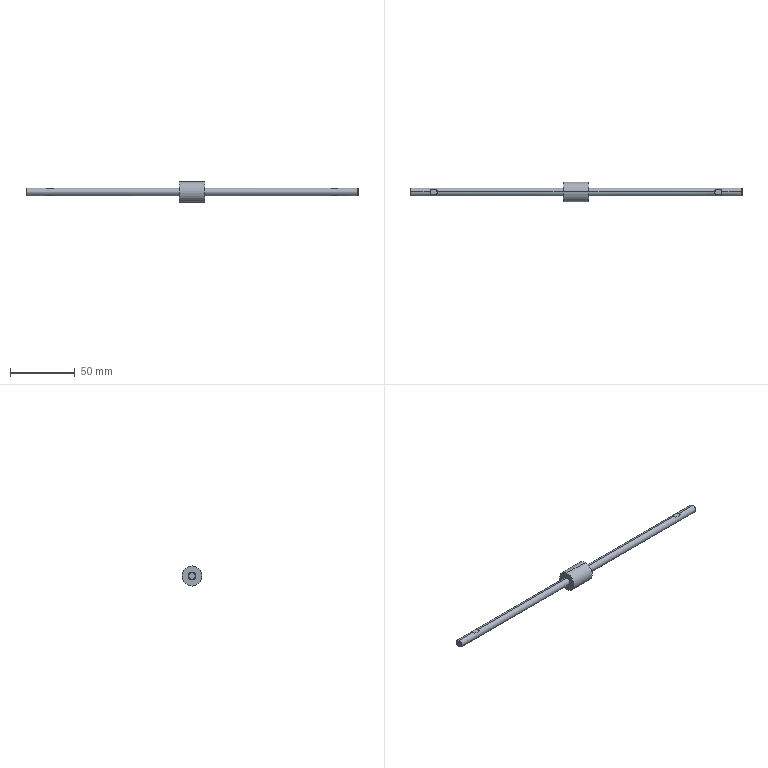Part | STEP file | _16MAD600Rod | 1 solid | 26 faces | box 256 x 15.5 x 15.5 mm | volume 10417 mm3 | plane 16 | cylinder 6 | cone 4 | commonest cylinder face diameters 6 x4 15.5 x2
STEP:
#1=CARTESIAN_POINT('',(118.,0.,3.));
#2=VERTEX_POINT('',#1);
#3=CARTESIAN_POINT('',(118.,0.,-3.));
#4=VERTEX_POINT('',#3);
#5=CARTESIAN_POINT('',(118.,0.,0.));
#6=DIRECTION('',(-1.,0.,0.));
#7=DIRECTION('',(0.,0.,1.));
#8=AXIS2_PLACEMENT_3D('',#5,#6,#7);
#9=CIRCLE('',#8,3.);
#10=EDGE_CURVE('',#2,#4,#9,.T.);
#11=ORIENTED_EDGE('',*,*,#10,.T.);
#12=CARTESIAN_POINT('',(21.3,0.,-3.));
#13=VERTEX_POINT('',#12);
#14=CARTESIAN_POINT('',(256.,0.,-3.));
#15=DIRECTION('',(-1.,0.,0.));
#16=VECTOR('',#15,1000.);
#17=LINE('',#14,#16);
#18=EDGE_CURVE('',#4,#13,#17,.T.);
#19=ORIENTED_EDGE('',*,*,#18,.T.);
#20=CARTESIAN_POINT('',(20.8,1.658,-2.5));
#21=VERTEX_POINT('',#20);
#22=CARTESIAN_POINT('',(21.3,0.,-3.));
#23=CARTESIAN_POINT('',(21.3,0.5942,-3.));
#24=CARTESIAN_POINT('',(21.128,1.163,-2.828));
#25=CARTESIAN_POINT('',(20.8,1.658,-2.5));
#26=(BOUNDED_CURVE()B_SPLINE_CURVE(3,(#22,#23,#24,#25),.UNSPECIFIED.,.F.,.F.)B_SPLINE_CURVE_WITH_KNOTS((4,4),(3.142,3.727),.UNSPECIFIED.)CURVE()GEOMETRIC_REPRESENTATION_ITEM()RATIONAL_B_SPLINE_CURVE((1.,0.9716,0.9716,1.))REPRESENTATION_ITEM(''));
#27=EDGE_CURVE('',#13,#21,#26,.T.);
#28=ORIENTED_EDGE('',*,*,#27,.T.);
#29=CARTESIAN_POINT('',(16.,1.658,-2.5));
#30=VERTEX_POINT('',#29);
#31=CARTESIAN_POINT('',(256.,1.658,-2.5));
#32=DIRECTION('',(-1.,0.,0.));
#33=VECTOR('',#32,1000.);
#34=LINE('',#31,#33);
#35=EDGE_CURVE('',#21,#30,#34,.T.);
#36=ORIENTED_EDGE('',*,*,#35,.T.);
#37=CARTESIAN_POINT('',(15.5,0.,-3.));
#38=VERTEX_POINT('',#37);
#39=CARTESIAN_POINT('',(16.,1.658,-2.5));
#40=CARTESIAN_POINT('',(15.672,1.163,-2.828));
#41=CARTESIAN_POINT('',(15.5,0.5942,-3.));
#42=CARTESIAN_POINT('',(15.5,0.,-3.));
#43=(BOUNDED_CURVE()B_SPLINE_CURVE(3,(#39,#40,#41,#42),.UNSPECIFIED.,.F.,.F.)B_SPLINE_CURVE_WITH_KNOTS((4,4),(5.697,6.283),.UNSPECIFIED.)CURVE()GEOMETRIC_REPRESENTATION_ITEM()RATIONAL_B_SPLINE_CURVE((1.,0.9716,0.9716,1.))REPRESENTATION_ITEM(''));
#44=EDGE_CURVE('',#30,#38,#43,.T.);
#45=ORIENTED_EDGE('',*,*,#44,.T.);
#46=CARTESIAN_POINT('',(0.6135,0.,-3.));
#47=VERTEX_POINT('',#46);
#48=CARTESIAN_POINT('',(256.,0.,-3.));
#49=DIRECTION('',(-1.,0.,0.));
#50=VECTOR('',#49,1000.);
#51=LINE('',#48,#50);
#52=EDGE_CURVE('',#38,#47,#51,.T.);
#53=ORIENTED_EDGE('',*,*,#52,.T.);
#54=CARTESIAN_POINT('',(0.6135,0.,3.));
#55=VERTEX_POINT('',#54);
#56=CARTESIAN_POINT('',(0.6135,0.,0.));
#57=DIRECTION('',(1.,0.,0.));
#58=DIRECTION('',(0.,0.,1.));
#59=AXIS2_PLACEMENT_3D('',#56,#57,#58);
#60=CIRCLE('',#59,3.);
#61=EDGE_CURVE('',#47,#55,#60,.T.);
#62=ORIENTED_EDGE('',*,*,#61,.T.);
#63=CARTESIAN_POINT('',(15.5,0.,3.));
#64=VERTEX_POINT('',#63);
#65=CARTESIAN_POINT('',(256.,0.,3.));
#66=DIRECTION('',(-1.,0.,0.));
#67=VECTOR('',#66,1000.);
#68=LINE('',#65,#67);
#69=EDGE_CURVE('',#64,#55,#68,.T.);
#70=ORIENTED_EDGE('',*,*,#69,.F.);
#71=CARTESIAN_POINT('',(16.,1.658,2.5));
#72=VERTEX_POINT('',#71);
#73=CARTESIAN_POINT('',(15.5,0.,3.));
#74=CARTESIAN_POINT('',(15.5,0.5942,3.));
#75=CARTESIAN_POINT('',(15.672,1.163,2.828));
#76=CARTESIAN_POINT('',(16.,1.658,2.5));
#77=(BOUNDED_CURVE()B_SPLINE_CURVE(3,(#73,#74,#75,#76),.UNSPECIFIED.,.F.,.F.)B_SPLINE_CURVE_WITH_KNOTS((4,4),(0.,0.5857),.UNSPECIFIED.)CURVE()GEOMETRIC_REPRESENTATION_ITEM()RATIONAL_B_SPLINE_CURVE((1.,0.9716,0.9716,1.))REPRESENTATION_ITEM(''));
#78=EDGE_CURVE('',#64,#72,#77,.T.);
#79=ORIENTED_EDGE('',*,*,#78,.T.);
#80=CARTESIAN_POINT('',(20.8,1.658,2.5));
#81=VERTEX_POINT('',#80);
#82=CARTESIAN_POINT('',(256.,1.658,2.5));
#83=DIRECTION('',(1.,0.,0.));
#84=VECTOR('',#83,1000.);
#85=LINE('',#82,#84);
#86=EDGE_CURVE('',#72,#81,#85,.T.);
#87=ORIENTED_EDGE('',*,*,#86,.T.);
#88=CARTESIAN_POINT('',(21.3,0.,3.));
#89=VERTEX_POINT('',#88);
#90=CARTESIAN_POINT('',(20.8,1.658,2.5));
#91=CARTESIAN_POINT('',(21.128,1.163,2.828));
#92=CARTESIAN_POINT('',(21.3,0.5942,3.));
#93=CARTESIAN_POINT('',(21.3,0.,3.));
#94=(BOUNDED_CURVE()B_SPLINE_CURVE(3,(#90,#91,#92,#93),.UNSPECIFIED.,.F.,.F.)B_SPLINE_CURVE_WITH_KNOTS((4,4),(2.556,3.142),.UNSPECIFIED.)CURVE()GEOMETRIC_REPRESENTATION_ITEM()RATIONAL_B_SPLINE_CURVE((1.,0.9716,0.9716,1.))REPRESENTATION_ITEM(''));
#95=EDGE_CURVE('',#81,#89,#94,.T.);
#96=ORIENTED_EDGE('',*,*,#95,.T.);
#97=CARTESIAN_POINT('',(256.,0.,3.));
#98=DIRECTION('',(-1.,0.,0.));
#99=VECTOR('',#98,1000.);
#100=LINE('',#97,#99);
#101=EDGE_CURVE('',#2,#89,#100,.T.);
#102=ORIENTED_EDGE('',*,*,#101,.F.);
#103=EDGE_LOOP('',(#11,#19,#28,#36,#45,#53,#62,#70,#79,#87,#96,#102));
#104=FACE_OUTER_BOUND('',#103,.T.);
#105=CARTESIAN_POINT('',(256.,0.,0.));
#106=DIRECTION('',(-1.,0.,0.));
#107=DIRECTION('',(0.,0.,1.));
#108=AXIS2_PLACEMENT_3D('',#105,#106,#107);
#109=CYLINDRICAL_SURFACE('',#108,3.);
#110=ADVANCED_FACE('',(#104),#109,.T.);
#111=CARTESIAN_POINT('',(0.,0.,-2.387));
#112=VERTEX_POINT('',#111);
#113=CARTESIAN_POINT('',(0.,0.,2.387));
#114=VERTEX_POINT('',#113);
#115=CARTESIAN_POINT('',(0.,0.,0.));
#116=DIRECTION('',(1.,0.,0.));
#117=DIRECTION('',(0.,0.,-1.));
#118=AXIS2_PLACEMENT_3D('',#115,#116,#117);
#119=CIRCLE('',#118,2.387);
#120=EDGE_CURVE('',#112,#114,#119,.T.);
#121=ORIENTED_EDGE('',*,*,#120,.T.);
#122=CARTESIAN_POINT('',(0.6135,0.,3.));
#123=DIRECTION('',(0.7071,0.,0.7071));
#124=VECTOR('',#123,1000.);
#125=LINE('',#122,#124);
#126=EDGE_CURVE('',#114,#55,#125,.T.);
#127=ORIENTED_EDGE('',*,*,#126,.T.);
#128=ORIENTED_EDGE('',*,*,#61,.F.);
#129=CARTESIAN_POINT('',(0.6135,0.,-3.));
#130=DIRECTION('',(0.7071,0.,-0.7071));
#131=VECTOR('',#130,1000.);
#132=LINE('',#129,#131);
#133=EDGE_CURVE('',#112,#47,#132,.T.);
#134=ORIENTED_EDGE('',*,*,#133,.F.);
#135=EDGE_LOOP('',(#121,#127,#128,#134));
#136=FACE_OUTER_BOUND('',#135,.T.);
#137=CARTESIAN_POINT('',(0.6135,0.,0.));
#138=DIRECTION('',(1.,0.,0.));
#139=DIRECTION('',(0.,0.,-1.));
#140=AXIS2_PLACEMENT_3D('',#137,#138,#139);
#141=CONICAL_SURFACE('',#140,3.,0.7854);
#142=ADVANCED_FACE('',(#136),#141,.T.);
#143=CARTESIAN_POINT('',(138.,0.,7.75));
#144=VERTEX_POINT('',#143);
#145=CARTESIAN_POINT('',(138.,0.,-7.75));
#146=VERTEX_POINT('',#145);
#147=CARTESIAN_POINT('',(138.,0.,0.));
#148=DIRECTION('',(-1.,0.,0.));
#149=DIRECTION('',(0.,0.,1.));
#150=AXIS2_PLACEMENT_3D('',#147,#148,#149);
#151=CIRCLE('',#150,7.75);
#152=EDGE_CURVE('',#144,#146,#151,.T.);
#153=ORIENTED_EDGE('',*,*,#152,.T.);
#154=CARTESIAN_POINT('',(118.,0.,-7.75));
#155=VERTEX_POINT('',#154);
#156=CARTESIAN_POINT('',(256.,0.,-7.75));
#157=DIRECTION('',(-1.,0.,0.));
#158=VECTOR('',#157,1000.);
#159=LINE('',#156,#158);
#160=EDGE_CURVE('',#146,#155,#159,.T.);
#161=ORIENTED_EDGE('',*,*,#160,.T.);
#162=CARTESIAN_POINT('',(118.,0.,7.75));
#163=VERTEX_POINT('',#162);
#164=CARTESIAN_POINT('',(118.,0.,0.));
#165=DIRECTION('',(1.,0.,0.));
#166=DIRECTION('',(0.,0.,1.));
#167=AXIS2_PLACEMENT_3D('',#164,#165,#166);
#168=CIRCLE('',#167,7.75);
#169=EDGE_CURVE('',#155,#163,#168,.T.);
#170=ORIENTED_EDGE('',*,*,#169,.T.);
#171=CARTESIAN_POINT('',(256.,0.,7.75));
#172=DIRECTION('',(-1.,0.,0.));
#173=VECTOR('',#172,1000.);
#174=LINE('',#171,#173);
#175=EDGE_CURVE('',#144,#163,#174,.T.);
#176=ORIENTED_EDGE('',*,*,#175,.F.);
#177=EDGE_LOOP('',(#153,#161,#170,#176));
#178=FACE_OUTER_BOUND('',#177,.T.);
#179=CARTESIAN_POINT('',(256.,0.,0.));
#180=DIRECTION('',(-1.,0.,0.));
#181=DIRECTION('',(0.,0.,1.));
#182=AXIS2_PLACEMENT_3D('',#179,#180,#181);
#183=CYLINDRICAL_SURFACE('',#182,7.75);
#184=ADVANCED_FACE('',(#178),#183,.T.);
#185=CARTESIAN_POINT('',(255.387,0.,3.));
#186=VERTEX_POINT('',#185);
#187=CARTESIAN_POINT('',(255.387,0.,-3.));
#188=VERTEX_POINT('',#187);
#189=CARTESIAN_POINT('',(255.387,0.,0.));
#190=DIRECTION('',(-1.,0.,0.));
#191=DIRECTION('',(0.,0.,1.));
#192=AXIS2_PLACEMENT_3D('',#189,#190,#191);
#193=CIRCLE('',#192,3.);
#194=EDGE_CURVE('',#186,#188,#193,.T.);
#195=ORIENTED_EDGE('',*,*,#194,.T.);
#196=CARTESIAN_POINT('',(240.5,0.,-3.));
#197=VERTEX_POINT('',#196);
#198=CARTESIAN_POINT('',(256.,0.,-3.));
#199=DIRECTION('',(-1.,0.,0.));
#200=VECTOR('',#199,1000.);
#201=LINE('',#198,#200);
#202=EDGE_CURVE('',#188,#197,#201,.T.);
#203=ORIENTED_EDGE('',*,*,#202,.T.);
#204=CARTESIAN_POINT('',(240.,1.658,-2.5));
#205=VERTEX_POINT('',#204);
#206=CARTESIAN_POINT('',(240.5,0.,-3.));
#207=CARTESIAN_POINT('',(240.5,0.5942,-3.));
#208=CARTESIAN_POINT('',(240.328,1.163,-2.828));
#209=CARTESIAN_POINT('',(240.,1.658,-2.5));
#210=(BOUNDED_CURVE()B_SPLINE_CURVE(3,(#206,#207,#208,#209),.UNSPECIFIED.,.F.,.F.)B_SPLINE_CURVE_WITH_KNOTS((4,4),(3.142,3.727),.UNSPECIFIED.)CURVE()GEOMETRIC_REPRESENTATION_ITEM()RATIONAL_B_SPLINE_CURVE((1.,0.9716,0.9716,1.))REPRESENTATION_ITEM(''));
#211=EDGE_CURVE('',#197,#205,#210,.T.);
#212=ORIENTED_EDGE('',*,*,#211,.T.);
#213=CARTESIAN_POINT('',(235.2,1.658,-2.5));
#214=VERTEX_POINT('',#213);
#215=CARTESIAN_POINT('',(256.,1.658,-2.5));
#216=DIRECTION('',(-1.,0.,0.));
#217=VECTOR('',#216,1000.);
#218=LINE('',#215,#217);
#219=EDGE_CURVE('',#205,#214,#218,.T.);
#220=ORIENTED_EDGE('',*,*,#219,.T.);
#221=CARTESIAN_POINT('',(234.7,0.,-3.));
#222=VERTEX_POINT('',#221);
#223=CARTESIAN_POINT('',(235.2,1.658,-2.5));
#224=CARTESIAN_POINT('',(234.872,1.163,-2.828));
#225=CARTESIAN_POINT('',(234.7,0.5942,-3.));
#226=CARTESIAN_POINT('',(234.7,0.,-3.));
#227=(BOUNDED_CURVE()B_SPLINE_CURVE(3,(#223,#224,#225,#226),.UNSPECIFIED.,.F.,.T.)B_SPLINE_CURVE_WITH_KNOTS((4,4),(5.697,6.283),.UNSPECIFIED.)CURVE()GEOMETRIC_REPRESENTATION_ITEM()RATIONAL_B_SPLINE_CURVE((1.,0.9716,0.9716,1.))REPRESENTATION_ITEM(''));
#228=EDGE_CURVE('',#214,#222,#227,.T.);
#229=ORIENTED_EDGE('',*,*,#228,.T.);
#230=CARTESIAN_POINT('',(138.,0.,-3.));
#231=VERTEX_POINT('',#230);
#232=CARTESIAN_POINT('',(256.,0.,-3.));
#233=DIRECTION('',(-1.,0.,0.));
#234=VECTOR('',#233,1000.);
#235=LINE('',#232,#234);
#236=EDGE_CURVE('',#222,#231,#235,.T.);
#237=ORIENTED_EDGE('',*,*,#236,.T.);
#238=CARTESIAN_POINT('',(138.,0.,3.));
#239=VERTEX_POINT('',#238);
#240=CARTESIAN_POINT('',(138.,0.,0.));
#241=DIRECTION('',(1.,0.,0.));
#242=DIRECTION('',(0.,0.,1.));
#243=AXIS2_PLACEMENT_3D('',#240,#241,#242);
#244=CIRCLE('',#243,3.);
#245=EDGE_CURVE('',#231,#239,#244,.T.);
#246=ORIENTED_EDGE('',*,*,#245,.T.);
#247=CARTESIAN_POINT('',(234.7,0.,3.));
#248=VERTEX_POINT('',#247);
#249=CARTESIAN_POINT('',(256.,0.,3.));
#250=DIRECTION('',(-1.,0.,0.));
#251=VECTOR('',#250,1000.);
#252=LINE('',#249,#251);
#253=EDGE_CURVE('',#248,#239,#252,.T.);
#254=ORIENTED_EDGE('',*,*,#253,.F.);
#255=CARTESIAN_POINT('',(235.2,1.658,2.5));
#256=VERTEX_POINT('',#255);
#257=CARTESIAN_POINT('',(234.7,0.,3.));
#258=CARTESIAN_POINT('',(234.7,0.5942,3.));
#259=CARTESIAN_POINT('',(234.872,1.163,2.828));
#260=CARTESIAN_POINT('',(235.2,1.658,2.5));
#261=(BOUNDED_CURVE()B_SPLINE_CURVE(3,(#257,#258,#259,#260),.UNSPECIFIED.,.F.,.F.)B_SPLINE_CURVE_WITH_KNOTS((4,4),(0.,0.5857),.UNSPECIFIED.)CURVE()GEOMETRIC_REPRESENTATION_ITEM()RATIONAL_B_SPLINE_CURVE((1.,0.9716,0.9716,1.))REPRESENTATION_ITEM(''));
#262=EDGE_CURVE('',#248,#256,#261,.T.);
#263=ORIENTED_EDGE('',*,*,#262,.T.);
#264=CARTESIAN_POINT('',(240.,1.658,2.5));
#265=VERTEX_POINT('',#264);
#266=CARTESIAN_POINT('',(256.,1.658,2.5));
#267=DIRECTION('',(1.,0.,0.));
#268=VECTOR('',#267,1000.);
#269=LINE('',#266,#268);
#270=EDGE_CURVE('',#256,#265,#269,.T.);
#271=ORIENTED_EDGE('',*,*,#270,.T.);
#272=CARTESIAN_POINT('',(240.5,0.,3.));
#273=VERTEX_POINT('',#272);
#274=CARTESIAN_POINT('',(240.,1.658,2.5));
#275=CARTESIAN_POINT('',(240.328,1.163,2.828));
#276=CARTESIAN_POINT('',(240.5,0.5942,3.));
#277=CARTESIAN_POINT('',(240.5,0.,3.));
#278=(BOUNDED_CURVE()B_SPLINE_CURVE(3,(#274,#275,#276,#277),.UNSPECIFIED.,.F.,.F.)B_SPLINE_CURVE_WITH_KNOTS((4,4),(2.556,3.142),.UNSPECIFIED.)CURVE()GEOMETRIC_REPRESENTATION_ITEM()RATIONAL_B_SPLINE_CURVE((1.,0.9716,0.9716,1.))REPRESENTATION_ITEM(''));
#279=EDGE_CURVE('',#265,#273,#278,.T.);
#280=ORIENTED_EDGE('',*,*,#279,.T.);
#281=CARTESIAN_POINT('',(256.,0.,3.));
#282=DIRECTION('',(-1.,0.,0.));
#283=VECTOR('',#282,1000.);
#284=LINE('',#281,#283);
#285=EDGE_CURVE('',#186,#273,#284,.T.);
#286=ORIENTED_EDGE('',*,*,#285,.F.);
#287=EDGE_LOOP('',(#195,#203,#212,#220,#229,#237,#246,#254,#263,#271,#280,#286));
#288=FACE_OUTER_BOUND('',#287,.T.);
#289=CARTESIAN_POINT('',(256.,0.,0.));
#290=DIRECTION('',(-1.,0.,0.));
#291=DIRECTION('',(0.,0.,1.));
#292=AXIS2_PLACEMENT_3D('',#289,#290,#291);
#293=CYLINDRICAL_SURFACE('',#292,3.);
#294=ADVANCED_FACE('',(#288),#293,.T.);
#295=CARTESIAN_POINT('',(256.,0.,2.386));
#296=VERTEX_POINT('',#295);
#297=CARTESIAN_POINT('',(256.,0.,-2.386));
#298=VERTEX_POINT('',#297);
#299=CARTESIAN_POINT('',(256.,0.,0.));
#300=DIRECTION('',(-1.,0.,0.));
#301=DIRECTION('',(0.,0.,1.));
#302=AXIS2_PLACEMENT_3D('',#299,#300,#301);
#303=CIRCLE('',#302,2.386);
#304=EDGE_CURVE('',#296,#298,#303,.T.);
#305=ORIENTED_EDGE('',*,*,#304,.T.);
#306=CARTESIAN_POINT('',(255.387,0.,-3.));
#307=DIRECTION('',(-0.7071,0.,-0.7071));
#308=VECTOR('',#307,1000.);
#309=LINE('',#306,#308);
#310=EDGE_CURVE('',#298,#188,#309,.T.);
#311=ORIENTED_EDGE('',*,*,#310,.T.);
#312=ORIENTED_EDGE('',*,*,#194,.F.);
#313=CARTESIAN_POINT('',(255.387,0.,3.));
#314=DIRECTION('',(-0.7071,0.,0.7071));
#315=VECTOR('',#314,1000.);
#316=LINE('',#313,#315);
#317=EDGE_CURVE('',#296,#186,#316,.T.);
#318=ORIENTED_EDGE('',*,*,#317,.F.);
#319=EDGE_LOOP('',(#305,#311,#312,#318));
#320=FACE_OUTER_BOUND('',#319,.T.);
#321=CARTESIAN_POINT('',(255.387,0.,0.));
#322=DIRECTION('',(-1.,0.,0.));
#323=DIRECTION('',(0.,0.,1.));
#324=AXIS2_PLACEMENT_3D('',#321,#322,#323);
#325=CONICAL_SURFACE('',#324,3.,0.7854);
#326=ADVANCED_FACE('',(#320),#325,.T.);
#327=ORIENTED_EDGE('',*,*,#18,.F.);
#328=CARTESIAN_POINT('',(118.,0.,0.));
#329=DIRECTION('',(-1.,0.,0.));
#330=DIRECTION('',(0.,0.,1.));
#331=AXIS2_PLACEMENT_3D('',#328,#329,#330);
#332=CIRCLE('',#331,3.);
#333=EDGE_CURVE('',#4,#2,#332,.T.);
#334=ORIENTED_EDGE('',*,*,#333,.T.);
#335=ORIENTED_EDGE('',*,*,#101,.T.);
#336=CARTESIAN_POINT('',(20.8,-1.658,2.5));
#337=VERTEX_POINT('',#336);
#338=CARTESIAN_POINT('',(21.3,0.,3.));
#339=CARTESIAN_POINT('',(21.3,-0.5942,3.));
#340=CARTESIAN_POINT('',(21.128,-1.163,2.828));
#341=CARTESIAN_POINT('',(20.8,-1.658,2.5));
#342=(BOUNDED_CURVE()B_SPLINE_CURVE(3,(#338,#339,#340,#341),.UNSPECIFIED.,.F.,.F.)B_SPLINE_CURVE_WITH_KNOTS((4,4),(3.142,3.727),.UNSPECIFIED.)CURVE()GEOMETRIC_REPRESENTATION_ITEM()RATIONAL_B_SPLINE_CURVE((1.,0.9716,0.9716,1.))REPRESENTATION_ITEM(''));
#343=EDGE_CURVE('',#89,#337,#342,.T.);
#344=ORIENTED_EDGE('',*,*,#343,.T.);
#345=CARTESIAN_POINT('',(16.,-1.658,2.5));
#346=VERTEX_POINT('',#345);
#347=CARTESIAN_POINT('',(256.,-1.658,2.5));
#348=DIRECTION('',(-1.,0.,0.));
#349=VECTOR('',#348,1000.);
#350=LINE('',#347,#349);
#351=EDGE_CURVE('',#337,#346,#350,.T.);
#352=ORIENTED_EDGE('',*,*,#351,.T.);
#353=CARTESIAN_POINT('',(16.,-1.658,2.5));
#354=CARTESIAN_POINT('',(15.672,-1.163,2.828));
#355=CARTESIAN_POINT('',(15.5,-0.5942,3.));
#356=CARTESIAN_POINT('',(15.5,0.,3.));
#357=(BOUNDED_CURVE()B_SPLINE_CURVE(3,(#353,#354,#355,#356),.UNSPECIFIED.,.F.,.F.)B_SPLINE_CURVE_WITH_KNOTS((4,4),(5.697,6.283),.UNSPECIFIED.)CURVE()GEOMETRIC_REPRESENTATION_ITEM()RATIONAL_B_SPLINE_CURVE((1.,0.9716,0.9716,1.))REPRESENTATION_ITEM(''));
#358=EDGE_CURVE('',#346,#64,#357,.T.);
#359=ORIENTED_EDGE('',*,*,#358,.T.);
#360=ORIENTED_EDGE('',*,*,#69,.T.);
#361=CARTESIAN_POINT('',(0.6135,0.,0.));
#362=DIRECTION('',(1.,0.,0.));
#363=DIRECTION('',(0.,0.,1.));
#364=AXIS2_PLACEMENT_3D('',#361,#362,#363);
#365=CIRCLE('',#364,3.);
#366=EDGE_CURVE('',#55,#47,#365,.T.);
#367=ORIENTED_EDGE('',*,*,#366,.T.);
#368=ORIENTED_EDGE('',*,*,#52,.F.);
#369=CARTESIAN_POINT('',(16.,-1.658,-2.5));
#370=VERTEX_POINT('',#369);
#371=CARTESIAN_POINT('',(15.5,0.,-3.));
#372=CARTESIAN_POINT('',(15.5,-0.5942,-3.));
#373=CARTESIAN_POINT('',(15.672,-1.163,-2.828));
#374=CARTESIAN_POINT('',(16.,-1.658,-2.5));
#375=(BOUNDED_CURVE()B_SPLINE_CURVE(3,(#371,#372,#373,#374),.UNSPECIFIED.,.F.,.T.)B_SPLINE_CURVE_WITH_KNOTS((4,4),(0.,0.5857),.UNSPECIFIED.)CURVE()GEOMETRIC_REPRESENTATION_ITEM()RATIONAL_B_SPLINE_CURVE((1.,0.9716,0.9716,1.))REPRESENTATION_ITEM(''));
#376=EDGE_CURVE('',#38,#370,#375,.T.);
#377=ORIENTED_EDGE('',*,*,#376,.T.);
#378=CARTESIAN_POINT('',(20.8,-1.658,-2.5));
#379=VERTEX_POINT('',#378);
#380=CARTESIAN_POINT('',(256.,-1.658,-2.5));
#381=DIRECTION('',(1.,0.,0.));
#382=VECTOR('',#381,1000.);
#383=LINE('',#380,#382);
#384=EDGE_CURVE('',#370,#379,#383,.T.);
#385=ORIENTED_EDGE('',*,*,#384,.T.);
#386=CARTESIAN_POINT('',(20.8,-1.658,-2.5));
#387=CARTESIAN_POINT('',(21.128,-1.163,-2.828));
#388=CARTESIAN_POINT('',(21.3,-0.5942,-3.));
#389=CARTESIAN_POINT('',(21.3,0.,-3.));
#390=(BOUNDED_CURVE()B_SPLINE_CURVE(3,(#386,#387,#388,#389),.UNSPECIFIED.,.F.,.F.)B_SPLINE_CURVE_WITH_KNOTS((4,4),(2.556,3.142),.UNSPECIFIED.)CURVE()GEOMETRIC_REPRESENTATION_ITEM()RATIONAL_B_SPLINE_CURVE((1.,0.9716,0.9716,1.))REPRESENTATION_ITEM(''));
#391=EDGE_CURVE('',#379,#13,#390,.T.);
#392=ORIENTED_EDGE('',*,*,#391,.T.);
#393=EDGE_LOOP('',(#327,#334,#335,#344,#352,#359,#360,#367,#368,#377,#385,#392));
#394=FACE_OUTER_BOUND('',#393,.T.);
#395=CARTESIAN_POINT('',(256.,0.,0.));
#396=DIRECTION('',(-1.,0.,0.));
#397=DIRECTION('',(0.,0.,1.));
#398=AXIS2_PLACEMENT_3D('',#395,#396,#397);
#399=CYLINDRICAL_SURFACE('',#398,3.);
#400=ADVANCED_FACE('',(#394),#399,.T.);
#401=ORIENTED_EDGE('',*,*,#86,.F.);
#402=CARTESIAN_POINT('',(16.,2.5,2.5));
#403=DIRECTION('',(0.,-1.,0.));
#404=VECTOR('',#403,1000.);
#405=LINE('',#402,#404);
#406=EDGE_CURVE('',#72,#346,#405,.T.);
#407=ORIENTED_EDGE('',*,*,#406,.T.);
#408=ORIENTED_EDGE('',*,*,#351,.F.);
#409=CARTESIAN_POINT('',(20.8,2.5,2.5));
#410=DIRECTION('',(0.,1.,0.));
#411=VECTOR('',#410,1000.);
#412=LINE('',#409,#411);
#413=EDGE_CURVE('',#337,#81,#412,.T.);
#414=ORIENTED_EDGE('',*,*,#413,.T.);
#415=EDGE_LOOP('',(#401,#407,#408,#414));
#416=FACE_OUTER_BOUND('',#415,.T.);
#417=CARTESIAN_POINT('',(20.8,2.5,2.5));
#418=DIRECTION('',(0.,0.,1.));
#419=DIRECTION('',(1.,0.,0.));
#420=AXIS2_PLACEMENT_3D('',#417,#418,#419);
#421=PLANE('',#420);
#422=ADVANCED_FACE('',(#416),#421,.T.);
#423=ORIENTED_EDGE('',*,*,#358,.F.);
#424=ORIENTED_EDGE('',*,*,#406,.F.);
#425=ORIENTED_EDGE('',*,*,#78,.F.);
#426=EDGE_LOOP('',(#423,#424,#425));
#427=FACE_OUTER_BOUND('',#426,.T.);
#428=CARTESIAN_POINT('',(16.,2.5,2.5));
#429=DIRECTION('',(0.7071,0.,0.7071));
#430=DIRECTION('',(0.7071,0.,-0.7071));
#431=AXIS2_PLACEMENT_3D('',#428,#429,#430);
#432=PLANE('',#431);
#433=ADVANCED_FACE('',(#427),#432,.T.);
#434=ORIENTED_EDGE('',*,*,#95,.F.);
#435=ORIENTED_EDGE('',*,*,#413,.F.);
#436=ORIENTED_EDGE('',*,*,#343,.F.);
#437=EDGE_LOOP('',(#434,#435,#436));
#438=FACE_OUTER_BOUND('',#437,.T.);
#439=CARTESIAN_POINT('',(30.3,2.5,12.));
#440=DIRECTION('',(-0.7071,0.,0.7071));
#441=DIRECTION('',(0.7071,0.,0.7071));
#442=AXIS2_PLACEMENT_3D('',#439,#440,#441);
#443=PLANE('',#442);
#444=ADVANCED_FACE('',(#438),#443,.T.);
#445=ORIENTED_EDGE('',*,*,#126,.F.);
#446=CARTESIAN_POINT('',(0.,0.,0.));
#447=DIRECTION('',(1.,0.,0.));
#448=DIRECTION('',(0.,0.,-1.));
#449=AXIS2_PLACEMENT_3D('',#446,#447,#448);
#450=CIRCLE('',#449,2.387);
#451=EDGE_CURVE('',#114,#112,#450,.T.);
#452=ORIENTED_EDGE('',*,*,#451,.T.);
#453=ORIENTED_EDGE('',*,*,#133,.T.);
#454=ORIENTED_EDGE('',*,*,#366,.F.);
#455=EDGE_LOOP('',(#445,#452,#453,#454));
#456=FACE_OUTER_BOUND('',#455,.T.);
#457=CARTESIAN_POINT('',(0.6135,0.,0.));
#458=DIRECTION('',(1.,0.,0.));
#459=DIRECTION('',(0.,0.,-1.));
#460=AXIS2_PLACEMENT_3D('',#457,#458,#459);
#461=CONICAL_SURFACE('',#460,3.,0.7854);
#462=ADVANCED_FACE('',(#456),#461,.T.);
#463=ORIENTED_EDGE('',*,*,#384,.F.);
#464=CARTESIAN_POINT('',(16.,2.5,-2.5));
#465=DIRECTION('',(0.,1.,0.));
#466=VECTOR('',#465,1000.);
#467=LINE('',#464,#466);
#468=EDGE_CURVE('',#370,#30,#467,.T.);
#469=ORIENTED_EDGE('',*,*,#468,.T.);
#470=ORIENTED_EDGE('',*,*,#35,.F.);
#471=CARTESIAN_POINT('',(20.8,2.5,-2.5));
#472=DIRECTION('',(0.,-1.,0.));
#473=VECTOR('',#472,1000.);
#474=LINE('',#471,#473);
#475=EDGE_CURVE('',#21,#379,#474,.T.);
#476=ORIENTED_EDGE('',*,*,#475,.T.);
#477=EDGE_LOOP('',(#463,#469,#470,#476));
#478=FACE_OUTER_BOUND('',#477,.T.);
#479=CARTESIAN_POINT('',(16.,2.5,-2.5));
#480=DIRECTION('',(0.,0.,-1.));
#481=DIRECTION('',(-1.,0.,0.));
#482=AXIS2_PLACEMENT_3D('',#479,#480,#481);
#483=PLANE('',#482);
#484=ADVANCED_FACE('',(#478),#483,.T.);
#485=ORIENTED_EDGE('',*,*,#391,.F.);
#486=ORIENTED_EDGE('',*,*,#475,.F.);
#487=ORIENTED_EDGE('',*,*,#27,.F.);
#488=EDGE_LOOP('',(#485,#486,#487));
#489=FACE_OUTER_BOUND('',#488,.T.);
#490=CARTESIAN_POINT('',(20.8,2.5,-2.5));
#491=DIRECTION('',(-0.7071,0.,-0.7071));
#492=DIRECTION('',(-0.7071,0.,0.7071));
#493=AXIS2_PLACEMENT_3D('',#490,#491,#492);
#494=PLANE('',#493);
#495=ADVANCED_FACE('',(#489),#494,.T.);
#496=ORIENTED_EDGE('',*,*,#44,.F.);
#497=ORIENTED_EDGE('',*,*,#468,.F.);
#498=ORIENTED_EDGE('',*,*,#376,.F.);
#499=EDGE_LOOP('',(#496,#497,#498));
#500=FACE_OUTER_BOUND('',#499,.T.);
#501=CARTESIAN_POINT('',(14.4,2.5,-4.1));
#502=DIRECTION('',(0.7071,0.,-0.7071));
#503=DIRECTION('',(-0.7071,0.,-0.7071));
#504=AXIS2_PLACEMENT_3D('',#501,#502,#503);
#505=PLANE('',#504);
#506=ADVANCED_FACE('',(#500),#505,.T.);
#507=ORIENTED_EDGE('',*,*,#10,.F.);
#508=ORIENTED_EDGE('',*,*,#333,.F.);
#509=EDGE_LOOP('',(#507,#508));
#510=FACE_BOUND('',#509,.T.);
#511=CARTESIAN_POINT('',(118.,0.,0.));
#512=DIRECTION('',(1.,0.,0.));
#513=DIRECTION('',(0.,0.,1.));
#514=AXIS2_PLACEMENT_3D('',#511,#512,#513);
#515=CIRCLE('',#514,7.75);
#516=EDGE_CURVE('',#163,#155,#515,.T.);
#517=ORIENTED_EDGE('',*,*,#516,.F.);
#518=ORIENTED_EDGE('',*,*,#169,.F.);
#519=EDGE_LOOP('',(#517,#518));
#520=FACE_OUTER_BOUND('',#519,.T.);
#521=CARTESIAN_POINT('',(118.,3.,0.));
#522=DIRECTION('',(1.,0.,0.));
#523=DIRECTION('',(0.,0.,-1.));
#524=AXIS2_PLACEMENT_3D('',#521,#522,#523);
#525=PLANE('',#524);
#526=ADVANCED_FACE('',(#510,#520),#525,.F.);
#527=ORIENTED_EDGE('',*,*,#120,.F.);
#528=ORIENTED_EDGE('',*,*,#451,.F.);
#529=EDGE_LOOP('',(#527,#528));
#530=FACE_OUTER_BOUND('',#529,.T.);
#531=CARTESIAN_POINT('',(0.,0.,0.));
#532=DIRECTION('',(1.,0.,0.));
#533=DIRECTION('',(0.,0.,-1.));
#534=AXIS2_PLACEMENT_3D('',#531,#532,#533);
#535=PLANE('',#534);
#536=ADVANCED_FACE('',(#530),#535,.F.);
#537=ORIENTED_EDGE('',*,*,#160,.F.);
#538=CARTESIAN_POINT('',(138.,0.,0.));
#539=DIRECTION('',(-1.,0.,0.));
#540=DIRECTION('',(0.,0.,1.));
#541=AXIS2_PLACEMENT_3D('',#538,#539,#540);
#542=CIRCLE('',#541,7.75);
#543=EDGE_CURVE('',#146,#144,#542,.T.);
#544=ORIENTED_EDGE('',*,*,#543,.T.);
#545=ORIENTED_EDGE('',*,*,#175,.T.);
#546=ORIENTED_EDGE('',*,*,#516,.T.);
#547=EDGE_LOOP('',(#537,#544,#545,#546));
#548=FACE_OUTER_BOUND('',#547,.T.);
#549=CARTESIAN_POINT('',(256.,0.,0.));
#550=DIRECTION('',(-1.,0.,0.));
#551=DIRECTION('',(0.,0.,1.));
#552=AXIS2_PLACEMENT_3D('',#549,#550,#551);
#553=CYLINDRICAL_SURFACE('',#552,7.75);
#554=ADVANCED_FACE('',(#548),#553,.T.);
#555=ORIENTED_EDGE('',*,*,#152,.F.);
#556=ORIENTED_EDGE('',*,*,#543,.F.);
#557=EDGE_LOOP('',(#555,#556));
#558=FACE_OUTER_BOUND('',#557,.T.);
#559=CARTESIAN_POINT('',(138.,0.,0.));
#560=DIRECTION('',(1.,0.,0.));
#561=DIRECTION('',(0.,0.,1.));
#562=AXIS2_PLACEMENT_3D('',#559,#560,#561);
#563=CIRCLE('',#562,3.);
#564=EDGE_CURVE('',#239,#231,#563,.T.);
#565=ORIENTED_EDGE('',*,*,#564,.F.);
#566=ORIENTED_EDGE('',*,*,#245,.F.);
#567=EDGE_LOOP('',(#565,#566));
#568=FACE_BOUND('',#567,.T.);
#569=CARTESIAN_POINT('',(138.,7.75,0.));
#570=DIRECTION('',(-1.,0.,0.));
#571=DIRECTION('',(0.,0.,1.));
#572=AXIS2_PLACEMENT_3D('',#569,#570,#571);
#573=PLANE('',#572);
#574=ADVANCED_FACE('',(#558,#568),#573,.F.);
#575=ORIENTED_EDGE('',*,*,#202,.F.);
#576=CARTESIAN_POINT('',(255.387,0.,0.));
#577=DIRECTION('',(-1.,0.,0.));
#578=DIRECTION('',(0.,0.,1.));
#579=AXIS2_PLACEMENT_3D('',#576,#577,#578);
#580=CIRCLE('',#579,3.);
#581=EDGE_CURVE('',#188,#186,#580,.T.);
#582=ORIENTED_EDGE('',*,*,#581,.T.);
#583=ORIENTED_EDGE('',*,*,#285,.T.);
#584=CARTESIAN_POINT('',(240.,-1.658,2.5));
#585=VERTEX_POINT('',#584);
#586=CARTESIAN_POINT('',(240.5,0.,3.));
#587=CARTESIAN_POINT('',(240.5,-0.5942,3.));
#588=CARTESIAN_POINT('',(240.328,-1.163,2.828));
#589=CARTESIAN_POINT('',(240.,-1.658,2.5));
#590=(BOUNDED_CURVE()B_SPLINE_CURVE(3,(#586,#587,#588,#589),.UNSPECIFIED.,.F.,.T.)B_SPLINE_CURVE_WITH_KNOTS((4,4),(3.142,3.727),.UNSPECIFIED.)CURVE()GEOMETRIC_REPRESENTATION_ITEM()RATIONAL_B_SPLINE_CURVE((1.,0.9716,0.9716,1.))REPRESENTATION_ITEM(''));
#591=EDGE_CURVE('',#273,#585,#590,.T.);
#592=ORIENTED_EDGE('',*,*,#591,.T.);
#593=CARTESIAN_POINT('',(235.2,-1.658,2.5));
#594=VERTEX_POINT('',#593);
#595=CARTESIAN_POINT('',(256.,-1.658,2.5));
#596=DIRECTION('',(-1.,0.,0.));
#597=VECTOR('',#596,1000.);
#598=LINE('',#595,#597);
#599=EDGE_CURVE('',#585,#594,#598,.T.);
#600=ORIENTED_EDGE('',*,*,#599,.T.);
#601=CARTESIAN_POINT('',(235.2,-1.658,2.5));
#602=CARTESIAN_POINT('',(234.872,-1.163,2.828));
#603=CARTESIAN_POINT('',(234.7,-0.5942,3.));
#604=CARTESIAN_POINT('',(234.7,0.,3.));
#605=(BOUNDED_CURVE()B_SPLINE_CURVE(3,(#601,#602,#603,#604),.UNSPECIFIED.,.F.,.F.)B_SPLINE_CURVE_WITH_KNOTS((4,4),(5.697,6.283),.UNSPECIFIED.)CURVE()GEOMETRIC_REPRESENTATION_ITEM()RATIONAL_B_SPLINE_CURVE((1.,0.9716,0.9716,1.))REPRESENTATION_ITEM(''));
#606=EDGE_CURVE('',#594,#248,#605,.T.);
#607=ORIENTED_EDGE('',*,*,#606,.T.);
#608=ORIENTED_EDGE('',*,*,#253,.T.);
#609=ORIENTED_EDGE('',*,*,#564,.T.);
#610=ORIENTED_EDGE('',*,*,#236,.F.);
#611=CARTESIAN_POINT('',(235.2,-1.658,-2.5));
#612=VERTEX_POINT('',#611);
#613=CARTESIAN_POINT('',(234.7,0.,-3.));
#614=CARTESIAN_POINT('',(234.7,-0.5942,-3.));
#615=CARTESIAN_POINT('',(234.872,-1.163,-2.828));
#616=CARTESIAN_POINT('',(235.2,-1.658,-2.5));
#617=(BOUNDED_CURVE()B_SPLINE_CURVE(3,(#613,#614,#615,#616),.UNSPECIFIED.,.F.,.T.)B_SPLINE_CURVE_WITH_KNOTS((4,4),(0.,0.5857),.UNSPECIFIED.)CURVE()GEOMETRIC_REPRESENTATION_ITEM()RATIONAL_B_SPLINE_CURVE((1.,0.9716,0.9716,1.))REPRESENTATION_ITEM(''));
#618=EDGE_CURVE('',#222,#612,#617,.T.);
#619=ORIENTED_EDGE('',*,*,#618,.T.);
#620=CARTESIAN_POINT('',(240.,-1.658,-2.5));
#621=VERTEX_POINT('',#620);
#622=CARTESIAN_POINT('',(256.,-1.658,-2.5));
#623=DIRECTION('',(1.,0.,0.));
#624=VECTOR('',#623,1000.);
#625=LINE('',#622,#624);
#626=EDGE_CURVE('',#612,#621,#625,.T.);
#627=ORIENTED_EDGE('',*,*,#626,.T.);
#628=CARTESIAN_POINT('',(240.,-1.658,-2.5));
#629=CARTESIAN_POINT('',(240.328,-1.163,-2.828));
#630=CARTESIAN_POINT('',(240.5,-0.5942,-3.));
#631=CARTESIAN_POINT('',(240.5,0.,-3.));
#632=(BOUNDED_CURVE()B_SPLINE_CURVE(3,(#628,#629,#630,#631),.UNSPECIFIED.,.F.,.F.)B_SPLINE_CURVE_WITH_KNOTS((4,4),(2.556,3.142),.UNSPECIFIED.)CURVE()GEOMETRIC_REPRESENTATION_ITEM()RATIONAL_B_SPLINE_CURVE((1.,0.9716,0.9716,1.))REPRESENTATION_ITEM(''));
#633=EDGE_CURVE('',#621,#197,#632,.T.);
#634=ORIENTED_EDGE('',*,*,#633,.T.);
#635=EDGE_LOOP('',(#575,#582,#583,#592,#600,#607,#608,#609,#610,#619,#627,#634));
#636=FACE_OUTER_BOUND('',#635,.T.);
#637=CARTESIAN_POINT('',(256.,0.,0.));
#638=DIRECTION('',(-1.,0.,0.));
#639=DIRECTION('',(0.,0.,1.));
#640=AXIS2_PLACEMENT_3D('',#637,#638,#639);
#641=CYLINDRICAL_SURFACE('',#640,3.);
#642=ADVANCED_FACE('',(#636),#641,.T.);
#643=ORIENTED_EDGE('',*,*,#626,.F.);
#644=CARTESIAN_POINT('',(235.2,2.5,-2.5));
#645=DIRECTION('',(0.,1.,0.));
#646=VECTOR('',#645,1000.);
#647=LINE('',#644,#646);
#648=EDGE_CURVE('',#612,#214,#647,.T.);
#649=ORIENTED_EDGE('',*,*,#648,.T.);
#650=ORIENTED_EDGE('',*,*,#219,.F.);
#651=CARTESIAN_POINT('',(240.,2.5,-2.5));
#652=DIRECTION('',(0.,-1.,0.));
#653=VECTOR('',#652,1000.);
#654=LINE('',#651,#653);
#655=EDGE_CURVE('',#205,#621,#654,.T.);
#656=ORIENTED_EDGE('',*,*,#655,.T.);
#657=EDGE_LOOP('',(#643,#649,#650,#656));
#658=FACE_OUTER_BOUND('',#657,.T.);
#659=CARTESIAN_POINT('',(235.2,2.5,-2.5));
#660=DIRECTION('',(0.,0.,-1.));
#661=DIRECTION('',(-1.,0.,0.));
#662=AXIS2_PLACEMENT_3D('',#659,#660,#661);
#663=PLANE('',#662);
#664=ADVANCED_FACE('',(#658),#663,.T.);
#665=ORIENTED_EDGE('',*,*,#633,.F.);
#666=ORIENTED_EDGE('',*,*,#655,.F.);
#667=ORIENTED_EDGE('',*,*,#211,.F.);
#668=EDGE_LOOP('',(#665,#666,#667));
#669=FACE_OUTER_BOUND('',#668,.T.);
#670=CARTESIAN_POINT('',(240.,2.5,-2.5));
#671=DIRECTION('',(-0.7071,0.,-0.7071));
#672=DIRECTION('',(-0.7071,0.,0.7071));
#673=AXIS2_PLACEMENT_3D('',#670,#671,#672);
#674=PLANE('',#673);
#675=ADVANCED_FACE('',(#669),#674,.T.);
#676=ORIENTED_EDGE('',*,*,#228,.F.);
#677=ORIENTED_EDGE('',*,*,#648,.F.);
#678=ORIENTED_EDGE('',*,*,#618,.F.);
#679=EDGE_LOOP('',(#676,#677,#678));
#680=FACE_OUTER_BOUND('',#679,.T.);
#681=CARTESIAN_POINT('',(225.7,2.5,-12.));
#682=DIRECTION('',(0.7071,0.,-0.7071));
#683=DIRECTION('',(-0.7071,0.,-0.7071));
#684=AXIS2_PLACEMENT_3D('',#681,#682,#683);
#685=PLANE('',#684);
#686=ADVANCED_FACE('',(#680),#685,.T.);
#687=ORIENTED_EDGE('',*,*,#279,.F.);
#688=CARTESIAN_POINT('',(240.,2.5,2.5));
#689=DIRECTION('',(0.,-1.,0.));
#690=VECTOR('',#689,1000.);
#691=LINE('',#688,#690);
#692=EDGE_CURVE('',#265,#585,#691,.T.);
#693=ORIENTED_EDGE('',*,*,#692,.T.);
#694=ORIENTED_EDGE('',*,*,#591,.F.);
#695=EDGE_LOOP('',(#687,#693,#694));
#696=FACE_OUTER_BOUND('',#695,.T.);
#697=CARTESIAN_POINT('',(241.6,2.5,4.1));
#698=DIRECTION('',(-0.7071,0.,0.7071));
#699=DIRECTION('',(0.7071,0.,0.7071));
#700=AXIS2_PLACEMENT_3D('',#697,#698,#699);
#701=PLANE('',#700);
#702=ADVANCED_FACE('',(#696),#701,.T.);
#703=ORIENTED_EDGE('',*,*,#270,.F.);
#704=CARTESIAN_POINT('',(235.2,2.5,2.5));
#705=DIRECTION('',(0.,-1.,0.));
#706=VECTOR('',#705,1000.);
#707=LINE('',#704,#706);
#708=EDGE_CURVE('',#256,#594,#707,.T.);
#709=ORIENTED_EDGE('',*,*,#708,.T.);
#710=ORIENTED_EDGE('',*,*,#599,.F.);
#711=ORIENTED_EDGE('',*,*,#692,.F.);
#712=EDGE_LOOP('',(#703,#709,#710,#711));
#713=FACE_OUTER_BOUND('',#712,.T.);
#714=CARTESIAN_POINT('',(240.,2.5,2.5));
#715=DIRECTION('',(0.,0.,1.));
#716=DIRECTION('',(1.,0.,0.));
#717=AXIS2_PLACEMENT_3D('',#714,#715,#716);
#718=PLANE('',#717);
#719=ADVANCED_FACE('',(#713),#718,.T.);
#720=ORIENTED_EDGE('',*,*,#606,.F.);
#721=ORIENTED_EDGE('',*,*,#708,.F.);
#722=ORIENTED_EDGE('',*,*,#262,.F.);
#723=EDGE_LOOP('',(#720,#721,#722));
#724=FACE_OUTER_BOUND('',#723,.T.);
#725=CARTESIAN_POINT('',(235.2,2.5,2.5));
#726=DIRECTION('',(0.7071,0.,0.7071));
#727=DIRECTION('',(0.7071,0.,-0.7071));
#728=AXIS2_PLACEMENT_3D('',#725,#726,#727);
#729=PLANE('',#728);
#730=ADVANCED_FACE('',(#724),#729,.T.);
#731=ORIENTED_EDGE('',*,*,#310,.F.);
#732=CARTESIAN_POINT('',(256.,0.,0.));
#733=DIRECTION('',(-1.,0.,0.));
#734=DIRECTION('',(0.,0.,1.));
#735=AXIS2_PLACEMENT_3D('',#732,#733,#734);
#736=CIRCLE('',#735,2.386);
#737=EDGE_CURVE('',#298,#296,#736,.T.);
#738=ORIENTED_EDGE('',*,*,#737,.T.);
#739=ORIENTED_EDGE('',*,*,#317,.T.);
#740=ORIENTED_EDGE('',*,*,#581,.F.);
#741=EDGE_LOOP('',(#731,#738,#739,#740));
#742=FACE_OUTER_BOUND('',#741,.T.);
#743=CARTESIAN_POINT('',(255.387,0.,0.));
#744=DIRECTION('',(-1.,0.,0.));
#745=DIRECTION('',(0.,0.,1.));
#746=AXIS2_PLACEMENT_3D('',#743,#744,#745);
#747=CONICAL_SURFACE('',#746,3.,0.7854);
#748=ADVANCED_FACE('',(#742),#747,.T.);
#749=ORIENTED_EDGE('',*,*,#304,.F.);
#750=ORIENTED_EDGE('',*,*,#737,.F.);
#751=EDGE_LOOP('',(#749,#750));
#752=FACE_OUTER_BOUND('',#751,.T.);
#753=CARTESIAN_POINT('',(256.,2.386,0.));
#754=DIRECTION('',(-1.,0.,0.));
#755=DIRECTION('',(0.,0.,1.));
#756=AXIS2_PLACEMENT_3D('',#753,#754,#755);
#757=PLANE('',#756);
#758=ADVANCED_FACE('',(#752),#757,.F.);
#759=CLOSED_SHELL('',(#110,#142,#184,#294,#326,#400,#422,#433,#444,#462,#484,#495,#506,#526,#536,#554,#574,#642,#664,#675,#686,#702,#719,#730,#748,#758));
#760=MANIFOLD_SOLID_BREP('',#759);
#761=CARTESIAN_POINT('',(0.,0.,0.));
#762=DIRECTION('',(0.,0.,1.));
#763=DIRECTION('',(1.,0.,0.));
#764=AXIS2_PLACEMENT_3D('',#761,#762,#763);
#765=(LENGTH_UNIT()NAMED_UNIT(*)SI_UNIT(.MILLI.,.METRE.));
#766=UNCERTAINTY_MEASURE_WITH_UNIT(LENGTH_MEASURE(0.00001),#765,'','');
#767=(NAMED_UNIT(*)PLANE_ANGLE_UNIT()SI_UNIT($,.RADIAN.));
#768=(NAMED_UNIT(*)SI_UNIT($,.STERADIAN.)SOLID_ANGLE_UNIT());
#769=(GEOMETRIC_REPRESENTATION_CONTEXT(3)GLOBAL_UNCERTAINTY_ASSIGNED_CONTEXT((#766))GLOBAL_UNIT_ASSIGNED_CONTEXT((#765,#767,#768))REPRESENTATION_CONTEXT('',''));
#770=ADVANCED_BREP_SHAPE_REPRESENTATION('',(#760,#764),#769);